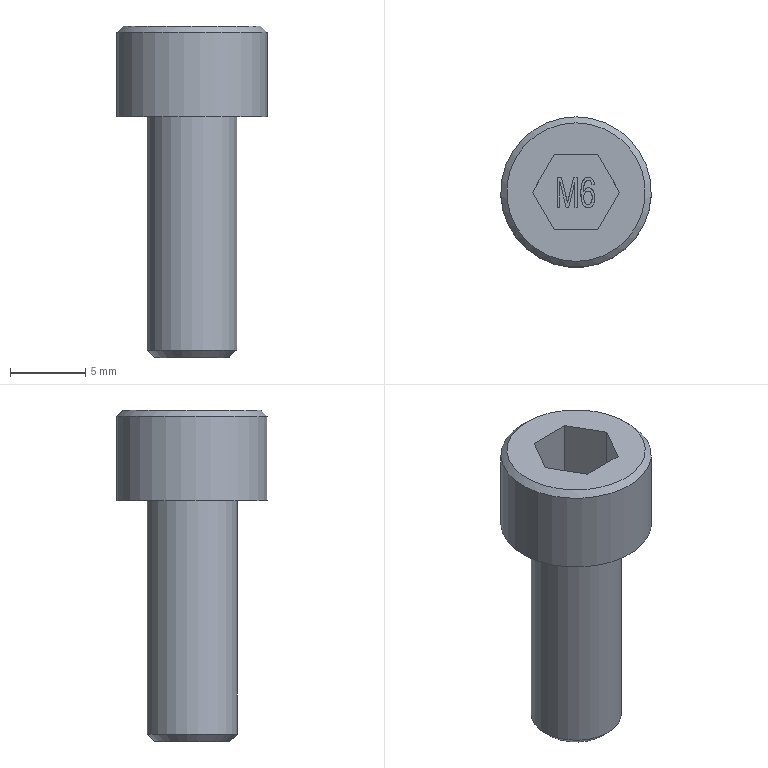Part | STEP file | EM10601600 | 1 solid | 38 faces | box 10 x 10 x 22 mm | volume 832.203 mm3 | plane 25 | other 9 | cylinder 2 | cone 2 | commonest cylinder face diameters 6 x1 10 x1